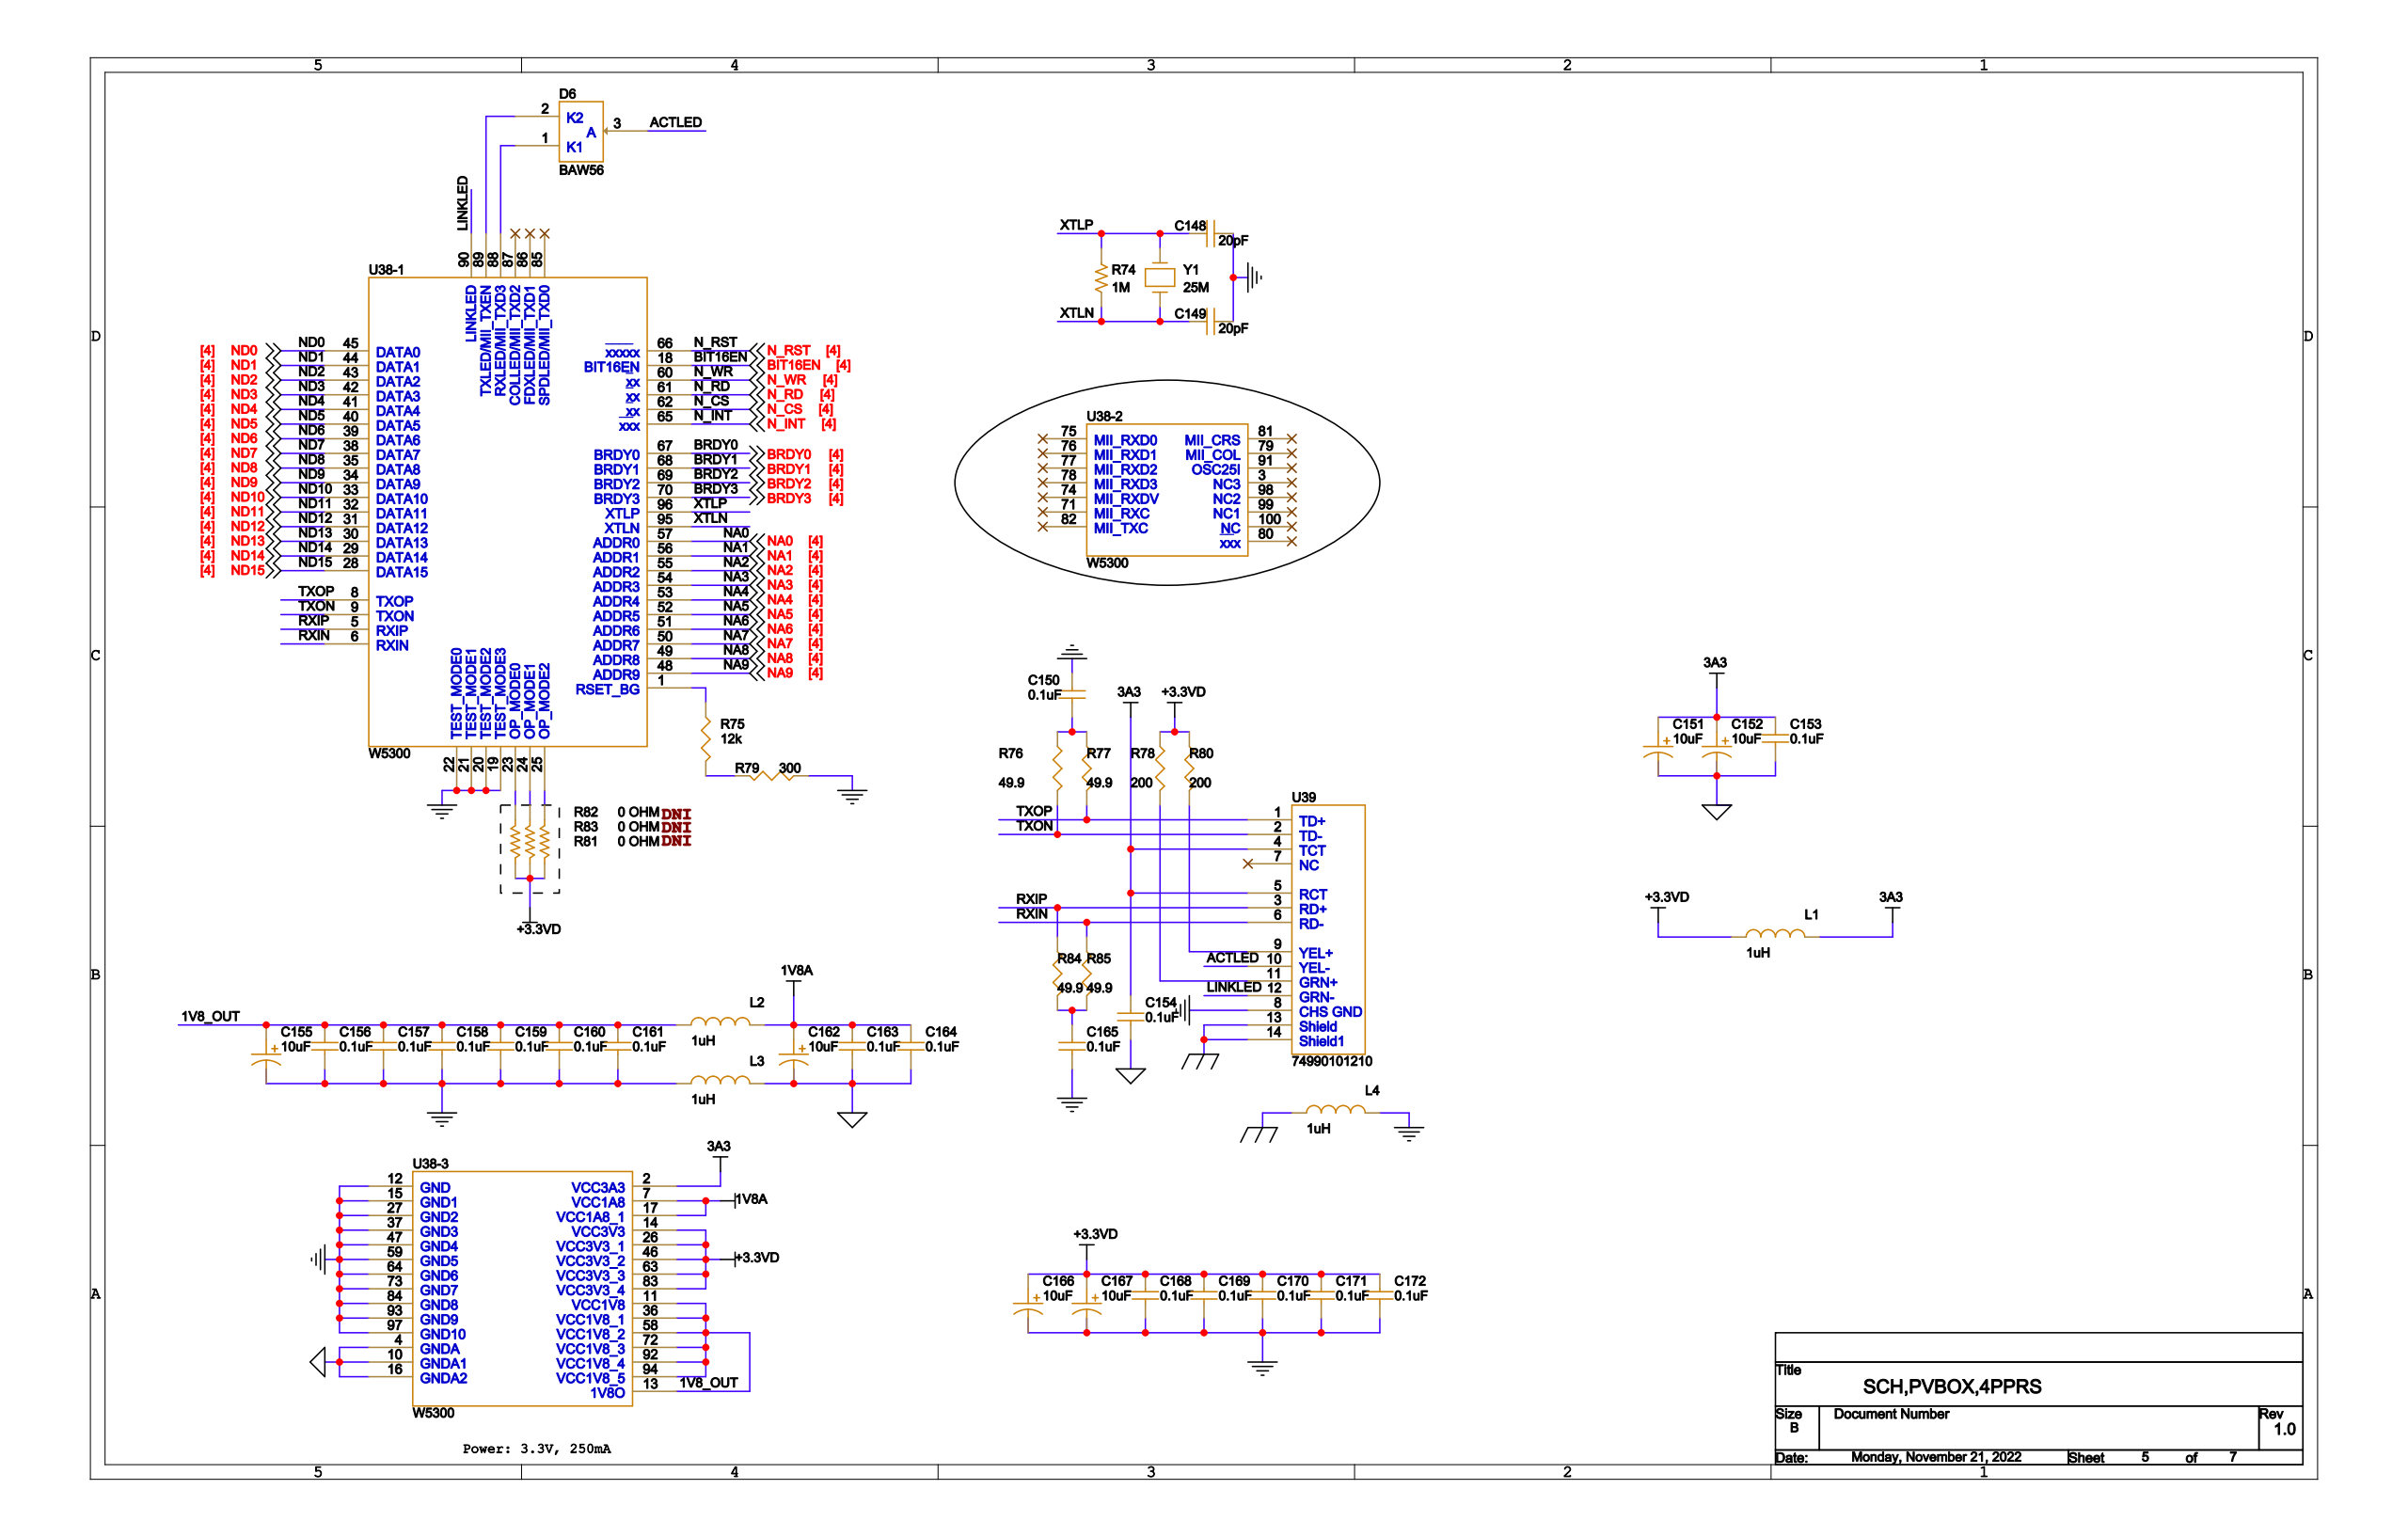Circuit board | Cadence Allegro | 405 parts | 254 nets | one sheet of the schematic
Parts on this sheet (reference | value | footprint):
C148 | C0603
C149 | C0603
C150 | C0603
C151 | C3528
C152 | C3528
C153 | C0402
C154 | C0603
C155 | C3528
C156 | C0402
C157 | C0402
C158 | C0402
C159 | C0402
C160 | C0402
C161 | C0402
C162 | C3528
C163 | C0402
C164 | C0402
C165 | C0603
C166 | C3528
C167 | C3528
C168 | C0402
C169 | C0402
C170 | C0402
C171 | C0402
C172 | C0402
D6 | SOT23
L1 | DO1608C
L2 | DO1608C
R74 | R0603
R76 | R0603
R77 | R0603
R78 | R0603
R79 | R0603
R80 | R0603
R81 | R0603
R82 | R0603
R83 | R0603
R84 | R0603
R85 | R0603
U39 | RJ45
Y1 | CO2-4R8X11R1-S
Nets of these parts (net: part-pin ...):
GND: C148-2 C149-2 C150-1 C155-2 C156-2 C157-2 C158-2 C159-2 C160-2 C161-2 C165-2 C166-2 C167-2 C168-2 C169-2 C170-2 C171-2 C172-2 R79-1 U39-8
+3.3VD: C166-1 C167-1 C168-1 C169-1 C170-1 C171-1 C172-1 L1-1 R78-1 R80-1 R81-1 R82-1 R83-1
N16966574: C150-2 R76-1 R77-1
3A3: C151-1 C152-1 C153-1 C154-1 L1-2 U39-4 U39-5
GND_SIGNAL: C151-2 C152-2 C153-2 C154-2 C162-2 C163-2 C164-2
N16966572: C165-1 R84-2 R85-2
XTLP: C148-1 R74-1 Y1-2
XTLN: C149-1 R74-2 Y1-1
1V8_OUT: C155-1 C156-1 C157-1 C158-1 C159-1 C160-1 C161-1 L2-1
1V8A: C162-1 C163-1 C164-1 L2-2
ACTLED: D6-3 U39-10
N16965158: D6-1
N16965161: D6-2
GND_EARTH: U39-13 U39-14
N16965024: R79-2
TXON: R76-2 U39-2
TXOP: R77-2 U39-1
RXIP: R84-1 U39-3
RXIN: R85-1 U39-6
N16966524: R78-2 U39-11
N16966520: R80-2 U39-9
N16965094: R81-2
N16965096: R82-2
N16965098: R83-2
LINKLED: U39-12